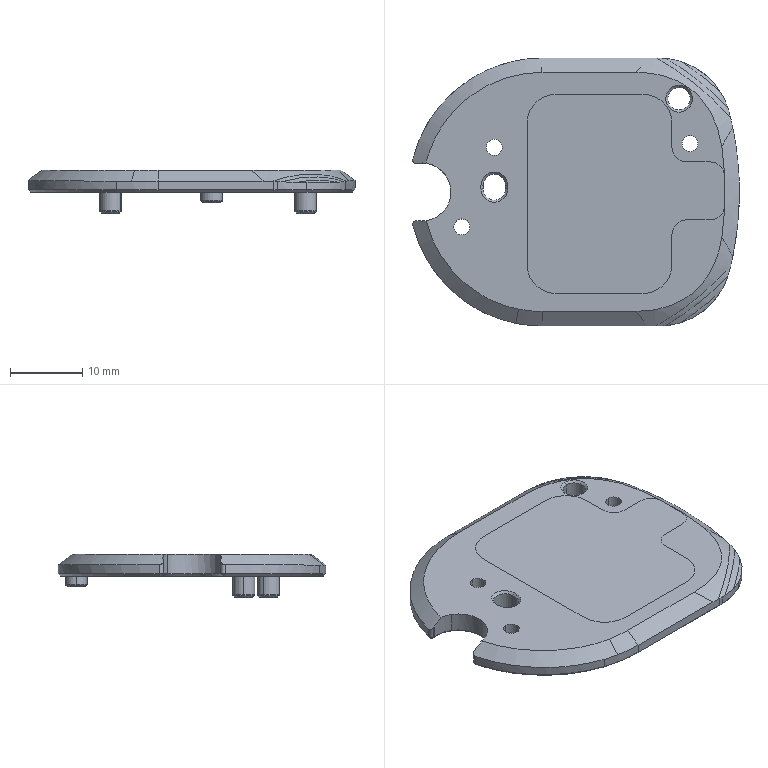NC program | NX | posted with a generic post | part box 45.101 x 36.973 x 6 mm
Lines 1 to 931 of 3161:
N10 G17 G21 G94 G90
(FLOOR_WALL_COPY , TOOL : D80)
N12 T19 M6
N14 G54
N16 G17 G0 G90 X-69.55 Y0. S6500 M3
N18 G43 Z30. H19
N20 Z3.
N22 G94 G1 Z0. F1500.
N24 X-64.55
N26 X64.55
N28 X69.55
N30 Z3.
N32 G0 Z30.
N34 M5
(ZLEVEL_PROFILE , TOOL : D10)
N36 T15 M6
N38 G54
N40 G17 G0 G90 X27.158 Y6.961 S9500 M3
N42 G43 Z30. H15
N44 Z1.5
N46 G94 G1 X27.257 Y6.402 Z1.47 F1000.
N48 X27.633 Y2.132 Z1.245
N50 X27.634 Y-2.155 Z1.021
N52 X27.259 Y-6.426 Z0.796
N54 X26.512 Y-10.647 Z0.571
N56 X26.081 Y-12.305 Z0.482
N58 X25.842 Y-13.227 Z0.432
N60 X24.998 Y-15.279 Z0.315
N62 X23.863 Y-17.185 Z0.199
N64 X22.461 Y-18.904 Z0.083
N66 X20.823 Y-20.4 Z-0.033
N68 X18.984 Y-21.641 Z-0.15
N70 X18.089 Y-22.081 Z-0.202
N72 X17.231 Y-22.495 Z-0.252
N74 X15.107 Y-23.182 Z-0.369
N76 X12.906 Y-23.549 Z-0.486
N78 X11.954 Y-23.576 Z-0.536
N80 X11.298 Y-23.585 Z-0.57
N82 X3.09 Z-1.
N84 X-5.774 Y-23.586 F3200.
N86 G2 X-27.477 Y-5.824 R23.6
N88 X-25.478 Y-0.018 R5.6
N90 X-27.478 Y5.788 R5.6
N92 X-4.605 Y23.585 R23.6
N94 G1 X11.247 Y23.586
N96 G2 X11.845 Y23.579 R23.599
N98 X26.079 Y12.281 R15.1
N100 X26.081 Y-12.305 R48.901
N102 X18.089 Y-22.081 R15.1
N104 X11.954 Y-23.576 R15.1
N106 G1 X11.298 Y-23.585
N108 X3.09
N110 X-4.652 Y-23.586 Z-1.135
N112 X-5.039 Y-23.582 Z-1.142
N114 X-5.426 Y-23.575 Z-1.149
N116 X-5.812 Y-23.559 Z-1.156
N118 X-6.198 Y-23.538 Z-1.162
N120 X-6.584 Y-23.51 Z-1.169
N122 X-6.969 Y-23.476 Z-1.176
N124 X-7.353 Y-23.435 Z-1.183
N126 X-7.737 Y-23.388 Z-1.189
N128 X-8.12 Y-23.335 Z-1.196
N130 X-8.503 Y-23.276 Z-1.203
N132 X-8.884 Y-23.21 Z-1.21
N134 X-9.264 Y-23.138 Z-1.216
N136 X-9.643 Y-23.059 Z-1.223
N138 X-10.021 Y-22.975 Z-1.23
N140 X-10.397 Y-22.885 Z-1.237
N142 X-10.771 Y-22.788 Z-1.243
N144 X-11.145 Y-22.687 Z-1.25
N146 X-11.511 Y-22.56 Z-1.257
N148 X-11.886 Y-22.462 Z-1.264
N150 X-12.253 Y-22.341 Z-1.27
N152 X-12.619 Y-22.213 Z-1.277
N154 X-12.982 Y-22.078 Z-1.284
N156 X-13.342 Y-21.938 Z-1.291
N158 X-13.701 Y-21.791 Z-1.297
N160 X-14.057 Y-21.639 Z-1.304
N162 X-14.41 Y-21.481 Z-1.311
N164 X-14.761 Y-21.318 Z-1.318
N166 X-15.109 Y-21.148 Z-1.325
N168 X-15.454 Y-20.973 Z-1.331
N170 X-15.796 Y-20.792 Z-1.338
N172 X-16.135 Y-20.606 Z-1.345
N174 X-16.472 Y-20.414 Z-1.352
N176 X-16.805 Y-20.216 Z-1.358
N178 X-17.134 Y-20.014 Z-1.365
N180 X-17.461 Y-19.805 Z-1.372
N182 X-17.783 Y-19.592 Z-1.379
N184 X-18.103 Y-19.373 Z-1.385
N186 X-18.418 Y-19.149 Z-1.392
N188 X-18.73 Y-18.92 Z-1.399
N190 X-19.039 Y-18.686 Z-1.406
N192 X-19.343 Y-18.446 Z-1.412
N194 X-19.643 Y-18.202 Z-1.419
N196 X-19.939 Y-17.953 Z-1.426
N198 X-20.232 Y-17.699 Z-1.433
N200 X-20.52 Y-17.44 Z-1.439
N202 X-20.803 Y-17.177 Z-1.446
N204 X-21.082 Y-16.909 Z-1.453
N206 X-21.357 Y-16.636 Z-1.46
N208 X-21.628 Y-16.359 Z-1.466
N210 X-21.893 Y-16.078 Z-1.473
N212 X-22.155 Y-15.792 Z-1.48
N214 X-22.411 Y-15.502 Z-1.487
N216 X-22.663 Y-15.208 Z-1.493
N218 X-22.909 Y-14.91 Z-1.5
N220 X-23.151 Y-14.607 Z-1.507
N222 X-23.388 Y-14.301 Z-1.514
N224 X-23.62 Y-13.991 Z-1.52
N226 X-23.846 Y-13.677 Z-1.527
N228 X-24.068 Y-13.36 Z-1.534
N230 X-24.284 Y-13.039 Z-1.541
N232 X-24.495 Y-12.714 Z-1.547
N234 X-24.701 Y-12.386 Z-1.554
N236 X-24.901 Y-12.055 Z-1.561
N238 X-25.096 Y-11.721 Z-1.568
N240 X-25.285 Y-11.383 Z-1.575
N242 X-25.469 Y-11.042 Z-1.581
N244 X-25.647 Y-10.698 Z-1.588
N246 X-25.819 Y-10.352 Z-1.595
N248 X-25.986 Y-10.003 Z-1.602
N250 X-26.147 Y-9.65 Z-1.608
N252 X-26.302 Y-9.296 Z-1.615
N254 X-26.451 Y-8.939 Z-1.622
N256 X-26.595 Y-8.579 Z-1.629
N258 X-26.732 Y-8.217 Z-1.635
N260 X-26.864 Y-7.853 Z-1.642
N262 X-26.989 Y-7.487 Z-1.649
N264 X-27.109 Y-7.119 Z-1.656
N266 X-27.222 Y-6.749 Z-1.662
N268 X-27.33 Y-6.377 Z-1.669
N270 X-27.431 Y-6.003 Z-1.676
N272 X-27.523 Y-5.627 Z-1.683
N274 X-27.592 Y-5.247 Z-1.689
N276 X-27.634 Y-4.862 Z-1.696
N278 X-27.649 Y-4.475 Z-1.703
N280 X-27.638 Y-4.088 Z-1.71
N282 X-27.6 Y-3.703 Z-1.716
N284 X-27.535 Y-3.322 Z-1.723
N286 X-27.445 Y-2.945 Z-1.73
N288 X-27.328 Y-2.576 Z-1.737
N290 X-27.186 Y-2.216 Z-1.743
N292 X-27.02 Y-1.867 Z-1.75
N294 X-26.83 Y-1.53 Z-1.757
N296 X-26.617 Y-1.206 Z-1.764
N298 X-26.383 Y-0.899 Z-1.77
N300 X-26.127 Y-0.608 Z-1.777
N302 X-25.852 Y-0.335 Z-1.784
N304 X-25.487 Y-0.009 Z-1.793
N306 X-25.697 Y0.161 Z-1.797
N308 X-25.982 Y0.423 Z-1.804
N310 X-26.248 Y0.704 Z-1.811
N312 X-26.494 Y1.003 Z-1.818
N314 X-26.718 Y1.318 Z-1.825
N316 X-26.921 Y1.648 Z-1.831
N318 X-27.1 Y1.991 Z-1.838
N320 X-27.255 Y2.345 Z-1.845
N322 X-27.386 Y2.71 Z-1.852
N324 X-27.49 Y3.082 Z-1.858
N326 X-27.569 Y3.461 Z-1.865
N328 X-27.622 Y3.844 Z-1.872
N330 X-27.647 Y4.231 Z-1.879
N332 Y4.618 Z-1.885
N334 X-27.619 Y5.004 Z-1.892
N336 X-27.565 Y5.387 Z-1.899
N338 X-27.484 Y5.765 Z-1.906
N340 X-27.386 Y6.14 Z-1.912
N342 X-27.282 Y6.513 Z-1.919
N344 X-27.172 Y6.884 Z-1.926
N346 X-27.056 Y7.253 Z-1.933
N348 X-26.934 Y7.62 Z-1.939
N350 X-26.805 Y7.986 Z-1.946
N352 X-26.671 Y8.349 Z-1.953
N354 X-26.531 Y8.71 Z-1.96
N356 X-26.385 Y9.068 Z-1.966
N358 X-26.233 Y9.424 Z-1.973
N360 X-26.075 Y9.778 Z-1.98
N362 X-25.912 Y10.128 Z-1.987
N364 X-25.743 Y10.477 Z-1.993
N366 X-25.568 Y10.822 Z-2.
N368 G2 X-4.605 Y23.585 R23.6
N370 G1 X11.247 Y23.586
N372 G2 X11.845 Y23.579 R23.599
N374 X26.079 Y12.281 R15.1
N376 X26.081 Y-12.305 R48.901
N378 X18.089 Y-22.081 R15.1
N380 X11.954 Y-23.576 R15.1
N382 G1 X11.298 Y-23.585
N384 X3.09
N386 X-4.652 Y-23.586 Z-2.135
N388 X-5.039 Y-23.582 Z-2.142
N390 X-5.426 Y-23.575 Z-2.149
N392 X-5.812 Y-23.559 Z-2.156
N394 X-6.198 Y-23.538 Z-2.162
N396 X-6.584 Y-23.51 Z-2.169
N398 X-6.969 Y-23.476 Z-2.176
N400 X-7.353 Y-23.435 Z-2.183
N402 X-7.737 Y-23.388 Z-2.189
N404 X-8.12 Y-23.335 Z-2.196
N406 X-8.503 Y-23.276 Z-2.203
N408 X-8.884 Y-23.21 Z-2.21
N410 X-9.264 Y-23.138 Z-2.216
N412 X-9.643 Y-23.059 Z-2.223
N414 X-10.021 Y-22.975 Z-2.23
N416 X-10.397 Y-22.885 Z-2.237
N418 X-10.771 Y-22.788 Z-2.243
N420 X-11.145 Y-22.687 Z-2.25
N422 X-11.511 Y-22.56 Z-2.257
N424 X-11.886 Y-22.462 Z-2.264
N426 X-12.253 Y-22.341 Z-2.27
N428 X-12.619 Y-22.213 Z-2.277
N430 X-12.982 Y-22.078 Z-2.284
N432 X-13.342 Y-21.938 Z-2.291
N434 X-13.701 Y-21.791 Z-2.297
N436 X-14.057 Y-21.639 Z-2.304
N438 X-14.41 Y-21.481 Z-2.311
N440 X-14.761 Y-21.318 Z-2.318
N442 X-15.109 Y-21.148 Z-2.325
N444 X-15.454 Y-20.973 Z-2.331
N446 X-15.796 Y-20.792 Z-2.338
N448 X-16.135 Y-20.606 Z-2.345
N450 X-16.472 Y-20.414 Z-2.352
N452 X-16.805 Y-20.216 Z-2.358
N454 X-17.134 Y-20.014 Z-2.365
N456 X-17.461 Y-19.805 Z-2.372
N458 X-17.783 Y-19.592 Z-2.379
N460 X-18.103 Y-19.373 Z-2.385
N462 X-18.418 Y-19.149 Z-2.392
N464 X-18.73 Y-18.92 Z-2.399
N466 X-19.039 Y-18.686 Z-2.406
N468 X-19.343 Y-18.446 Z-2.412
N470 X-19.643 Y-18.202 Z-2.419
N472 X-19.939 Y-17.953 Z-2.426
N474 X-20.232 Y-17.699 Z-2.433
N476 X-20.52 Y-17.44 Z-2.439
N478 X-20.803 Y-17.177 Z-2.446
N480 X-21.082 Y-16.909 Z-2.453
N482 X-21.357 Y-16.636 Z-2.46
N484 X-21.628 Y-16.359 Z-2.466
N486 X-21.893 Y-16.078 Z-2.473
N488 X-22.155 Y-15.792 Z-2.48
N490 X-22.411 Y-15.502 Z-2.487
N492 X-22.663 Y-15.208 Z-2.493
N494 X-22.909 Y-14.91 Z-2.5
N496 X-23.151 Y-14.607 Z-2.507
N498 X-23.388 Y-14.301 Z-2.514
N500 X-23.62 Y-13.991 Z-2.52
N502 X-23.846 Y-13.677 Z-2.527
N504 X-24.068 Y-13.36 Z-2.534
N506 X-24.284 Y-13.039 Z-2.541
N508 X-24.495 Y-12.714 Z-2.547
N510 X-24.701 Y-12.386 Z-2.554
N512 X-24.901 Y-12.055 Z-2.561
N514 X-25.096 Y-11.721 Z-2.568
N516 X-25.285 Y-11.383 Z-2.575
N518 X-25.469 Y-11.042 Z-2.581
N520 X-25.647 Y-10.698 Z-2.588
N522 X-25.819 Y-10.352 Z-2.595
N524 X-25.986 Y-10.003 Z-2.602
N526 X-26.147 Y-9.65 Z-2.608
N528 X-26.302 Y-9.296 Z-2.615
N530 X-26.451 Y-8.939 Z-2.622
N532 X-26.595 Y-8.579 Z-2.629
N534 X-26.732 Y-8.217 Z-2.635
N536 X-26.864 Y-7.853 Z-2.642
N538 X-26.989 Y-7.487 Z-2.649
N540 X-27.109 Y-7.119 Z-2.656
N542 X-27.222 Y-6.749 Z-2.662
N544 X-27.33 Y-6.377 Z-2.669
N546 X-27.431 Y-6.003 Z-2.676
N548 X-27.523 Y-5.627 Z-2.683
N550 X-27.592 Y-5.247 Z-2.689
N552 X-27.634 Y-4.862 Z-2.696
N554 X-27.649 Y-4.475 Z-2.703
N556 X-27.638 Y-4.088 Z-2.71
N558 X-27.6 Y-3.703 Z-2.716
N560 X-27.535 Y-3.322 Z-2.723
N562 X-27.445 Y-2.945 Z-2.73
N564 X-27.328 Y-2.576 Z-2.737
N566 X-27.186 Y-2.216 Z-2.743
N568 X-27.02 Y-1.867 Z-2.75
N570 X-26.83 Y-1.53 Z-2.757
N572 X-26.617 Y-1.206 Z-2.764
N574 X-26.383 Y-0.899 Z-2.77
N576 X-26.127 Y-0.608 Z-2.777
N578 X-25.852 Y-0.335 Z-2.784
N580 X-25.487 Y-0.009 Z-2.793
N582 X-25.697 Y0.161 Z-2.797
N584 X-25.982 Y0.423 Z-2.804
N586 X-26.248 Y0.704 Z-2.811
N588 X-26.494 Y1.003 Z-2.818
N590 X-26.718 Y1.318 Z-2.825
N592 X-26.921 Y1.648 Z-2.831
N594 X-27.1 Y1.991 Z-2.838
N596 X-27.255 Y2.345 Z-2.845
N598 X-27.386 Y2.71 Z-2.852
N600 X-27.49 Y3.082 Z-2.858
N602 X-27.569 Y3.461 Z-2.865
N604 X-27.622 Y3.844 Z-2.872
N606 X-27.647 Y4.231 Z-2.879
N608 Y4.618 Z-2.885
N610 X-27.619 Y5.004 Z-2.892
N612 X-27.565 Y5.387 Z-2.899
N614 X-27.484 Y5.765 Z-2.906
N616 X-27.386 Y6.14 Z-2.912
N618 X-27.282 Y6.513 Z-2.919
N620 X-27.172 Y6.884 Z-2.926
N622 X-27.056 Y7.253 Z-2.933
N624 X-26.934 Y7.62 Z-2.939
N626 X-26.805 Y7.986 Z-2.946
N628 X-26.671 Y8.349 Z-2.953
N630 X-26.531 Y8.71 Z-2.96
N632 X-26.385 Y9.068 Z-2.966
N634 X-26.233 Y9.424 Z-2.973
N636 X-26.075 Y9.778 Z-2.98
N638 X-25.912 Y10.128 Z-2.987
N640 X-25.743 Y10.477 Z-2.993
N642 X-25.568 Y10.822 Z-3.
N644 G2 X-4.605 Y23.585 R23.6
N646 G1 X11.247 Y23.586
N648 G2 X11.845 Y23.579 R23.599
N650 X26.079 Y12.281 R15.1
N652 X26.081 Y-12.305 R48.901
N654 X18.089 Y-22.081 R15.1
N656 X11.954 Y-23.576 R15.1
N658 G1 X11.298 Y-23.585
N660 X3.09
N662 X-4.652 Y-23.586 Z-3.135
N664 X-5.039 Y-23.582 Z-3.142
N666 X-5.426 Y-23.575 Z-3.149
N668 X-5.812 Y-23.559 Z-3.156
N670 X-6.198 Y-23.538 Z-3.162
N672 X-6.584 Y-23.51 Z-3.169
N674 X-6.969 Y-23.476 Z-3.176
N676 X-7.353 Y-23.435 Z-3.183
N678 X-7.737 Y-23.388 Z-3.189
N680 X-8.12 Y-23.335 Z-3.196
N682 X-8.503 Y-23.276 Z-3.203
N684 X-8.884 Y-23.21 Z-3.21
N686 X-9.264 Y-23.138 Z-3.216
N688 X-9.643 Y-23.059 Z-3.223
N690 X-10.021 Y-22.975 Z-3.23
N692 X-10.397 Y-22.885 Z-3.237
N694 X-10.771 Y-22.788 Z-3.243
N696 X-11.145 Y-22.687 Z-3.25
N698 X-11.511 Y-22.56 Z-3.257
N700 X-11.886 Y-22.462 Z-3.264
N702 X-12.253 Y-22.341 Z-3.27
N704 X-12.619 Y-22.213 Z-3.277
N706 X-12.982 Y-22.078 Z-3.284
N708 X-13.342 Y-21.938 Z-3.291
N710 X-13.701 Y-21.791 Z-3.297
N712 X-14.057 Y-21.639 Z-3.304
N714 X-14.41 Y-21.481 Z-3.311
N716 X-14.761 Y-21.318 Z-3.318
N718 X-15.109 Y-21.148 Z-3.325
N720 X-15.454 Y-20.973 Z-3.331
N722 X-15.796 Y-20.792 Z-3.338
N724 X-16.135 Y-20.606 Z-3.345
N726 X-16.472 Y-20.414 Z-3.352
N728 X-16.805 Y-20.216 Z-3.358
N730 X-17.134 Y-20.014 Z-3.365
N732 X-17.461 Y-19.805 Z-3.372
N734 X-17.783 Y-19.592 Z-3.379
N736 X-18.103 Y-19.373 Z-3.385
N738 X-18.418 Y-19.149 Z-3.392
N740 X-18.73 Y-18.92 Z-3.399
N742 X-19.039 Y-18.686 Z-3.406
N744 X-19.343 Y-18.446 Z-3.412
N746 X-19.643 Y-18.202 Z-3.419
N748 X-19.939 Y-17.953 Z-3.426
N750 X-20.232 Y-17.699 Z-3.433
N752 X-20.52 Y-17.44 Z-3.439
N754 X-20.803 Y-17.177 Z-3.446
N756 X-21.082 Y-16.909 Z-3.453
N758 X-21.357 Y-16.636 Z-3.46
N760 X-21.628 Y-16.359 Z-3.466
N762 X-21.893 Y-16.078 Z-3.473
N764 X-22.155 Y-15.792 Z-3.48
N766 X-22.411 Y-15.502 Z-3.487
N768 X-22.663 Y-15.208 Z-3.493
N770 X-22.909 Y-14.91 Z-3.5
N772 X-23.151 Y-14.607 Z-3.507
N774 X-23.388 Y-14.301 Z-3.514
N776 X-23.62 Y-13.991 Z-3.52
N778 X-23.846 Y-13.677 Z-3.527
N780 X-24.068 Y-13.36 Z-3.534
N782 X-24.284 Y-13.039 Z-3.541
N784 X-24.495 Y-12.714 Z-3.547
N786 X-24.701 Y-12.386 Z-3.554
N788 X-24.901 Y-12.055 Z-3.561
N790 X-25.096 Y-11.721 Z-3.568
N792 X-25.285 Y-11.383 Z-3.575
N794 X-25.469 Y-11.042 Z-3.581
N796 X-25.647 Y-10.698 Z-3.588
N798 X-25.819 Y-10.352 Z-3.595
N800 X-25.986 Y-10.003 Z-3.602
N802 X-26.147 Y-9.65 Z-3.608
N804 X-26.302 Y-9.296 Z-3.615
N806 X-26.451 Y-8.939 Z-3.622
N808 X-26.595 Y-8.579 Z-3.629
N810 X-26.732 Y-8.217 Z-3.635
N812 X-26.864 Y-7.853 Z-3.642
N814 X-26.989 Y-7.487 Z-3.649
N816 X-27.109 Y-7.119 Z-3.656
N818 X-27.222 Y-6.749 Z-3.662
N820 X-27.33 Y-6.377 Z-3.669
N822 X-27.431 Y-6.003 Z-3.676
N824 X-27.523 Y-5.627 Z-3.683
N826 X-27.592 Y-5.247 Z-3.689
N828 X-27.634 Y-4.862 Z-3.696
N830 X-27.649 Y-4.475 Z-3.703
N832 X-27.638 Y-4.088 Z-3.71
N834 X-27.6 Y-3.703 Z-3.716
N836 X-27.535 Y-3.322 Z-3.723
N838 X-27.445 Y-2.945 Z-3.73
N840 X-27.328 Y-2.576 Z-3.737
N842 X-27.186 Y-2.216 Z-3.743
N844 X-27.02 Y-1.867 Z-3.75
N846 X-26.83 Y-1.53 Z-3.757
N848 X-26.617 Y-1.206 Z-3.764
N850 X-26.383 Y-0.899 Z-3.77
N852 X-26.127 Y-0.608 Z-3.777
N854 X-25.852 Y-0.335 Z-3.784
N856 X-25.487 Y-0.009 Z-3.793
N858 X-25.697 Y0.161 Z-3.797
N860 X-25.982 Y0.423 Z-3.804
N862 X-26.248 Y0.704 Z-3.811
N864 X-26.494 Y1.003 Z-3.818
N866 X-26.718 Y1.318 Z-3.825
N868 X-26.921 Y1.648 Z-3.831
N870 X-27.1 Y1.991 Z-3.838
N872 X-27.255 Y2.345 Z-3.845
N874 X-27.386 Y2.71 Z-3.852
N876 X-27.49 Y3.082 Z-3.858
N878 X-27.569 Y3.461 Z-3.865
N880 X-27.622 Y3.844 Z-3.872
N882 X-27.647 Y4.231 Z-3.879
N884 Y4.618 Z-3.885
N886 X-27.619 Y5.004 Z-3.892
N888 X-27.565 Y5.387 Z-3.899
N890 X-27.484 Y5.765 Z-3.906
N892 X-27.386 Y6.14 Z-3.912
N894 X-27.282 Y6.513 Z-3.919
N896 X-27.172 Y6.884 Z-3.926
N898 X-27.056 Y7.253 Z-3.933
N900 X-26.934 Y7.62 Z-3.939
N902 X-26.805 Y7.986 Z-3.946
N904 X-26.671 Y8.349 Z-3.953
N906 X-26.531 Y8.71 Z-3.96
N908 X-26.385 Y9.068 Z-3.966
N910 X-26.233 Y9.424 Z-3.973
N912 X-26.075 Y9.778 Z-3.98
N914 X-25.912 Y10.128 Z-3.987
N916 X-25.743 Y10.477 Z-3.993
N918 X-25.568 Y10.822 Z-4.
N920 G2 X-4.605 Y23.585 R23.6
N922 G1 X11.247 Y23.586
N924 G2 X11.845 Y23.579 R23.599
N926 X26.079 Y12.281 R15.1
N928 X26.081 Y-12.305 R48.901
N930 X18.089 Y-22.081 R15.1
N932 X11.954 Y-23.576 R15.1
N934 G1 X11.298 Y-23.585
N936 X3.09
N938 X-4.652 Y-23.586 Z-4.135
N940 X-5.039 Y-23.582 Z-4.142
N942 X-5.426 Y-23.575 Z-4.149
N944 X-5.812 Y-23.559 Z-4.156
N946 X-6.198 Y-23.538 Z-4.162
N948 X-6.584 Y-23.51 Z-4.169
N950 X-6.969 Y-23.476 Z-4.176
N952 X-7.353 Y-23.435 Z-4.183
N954 X-7.737 Y-23.388 Z-4.189
N956 X-8.12 Y-23.335 Z-4.196
N958 X-8.503 Y-23.276 Z-4.203
N960 X-8.884 Y-23.21 Z-4.21
N962 X-9.264 Y-23.138 Z-4.216
N964 X-9.643 Y-23.059 Z-4.223
N966 X-10.021 Y-22.975 Z-4.23
N968 X-10.397 Y-22.885 Z-4.237
N970 X-10.771 Y-22.788 Z-4.243
N972 X-11.145 Y-22.687 Z-4.25
N974 X-11.511 Y-22.56 Z-4.257
N976 X-11.886 Y-22.462 Z-4.264
N978 X-12.253 Y-22.341 Z-4.27
N980 X-12.619 Y-22.213 Z-4.277
N982 X-12.982 Y-22.078 Z-4.284
N984 X-13.342 Y-21.938 Z-4.291
N986 X-13.701 Y-21.791 Z-4.297
N988 X-14.057 Y-21.639 Z-4.304
N990 X-14.41 Y-21.481 Z-4.311
N992 X-14.761 Y-21.318 Z-4.318
N994 X-15.109 Y-21.148 Z-4.325
N996 X-15.454 Y-20.973 Z-4.331
N998 X-15.796 Y-20.792 Z-4.338
N1000 X-16.135 Y-20.606 Z-4.345
N1002 X-16.472 Y-20.414 Z-4.352
N1004 X-16.805 Y-20.216 Z-4.358
N1006 X-17.134 Y-20.014 Z-4.365
N1008 X-17.461 Y-19.805 Z-4.372
N1010 X-17.783 Y-19.592 Z-4.379
N1012 X-18.103 Y-19.373 Z-4.385
N1014 X-18.418 Y-19.149 Z-4.392
N1016 X-18.73 Y-18.92 Z-4.399
N1018 X-19.039 Y-18.686 Z-4.406
N1020 X-19.343 Y-18.446 Z-4.412
N1022 X-19.643 Y-18.202 Z-4.419
N1024 X-19.939 Y-17.953 Z-4.426
N1026 X-20.232 Y-17.699 Z-4.433
N1028 X-20.52 Y-17.44 Z-4.439
N1030 X-20.803 Y-17.177 Z-4.446
N1032 X-21.082 Y-16.909 Z-4.453
N1034 X-21.357 Y-16.636 Z-4.46
N1036 X-21.628 Y-16.359 Z-4.466
N1038 X-21.893 Y-16.078 Z-4.473
N1040 X-22.155 Y-15.792 Z-4.48
N1042 X-22.411 Y-15.502 Z-4.487
N1044 X-22.663 Y-15.208 Z-4.493
N1046 X-22.909 Y-14.91 Z-4.5
N1048 X-23.151 Y-14.607 Z-4.507
N1050 X-23.388 Y-14.301 Z-4.514
N1052 X-23.62 Y-13.991 Z-4.52
N1054 X-23.846 Y-13.677 Z-4.527
N1056 X-24.068 Y-13.36 Z-4.534
N1058 X-24.284 Y-13.039 Z-4.541
N1060 X-24.495 Y-12.714 Z-4.547
N1062 X-24.701 Y-12.386 Z-4.554
N1064 X-24.901 Y-12.055 Z-4.561
N1066 X-25.096 Y-11.721 Z-4.568
N1068 X-25.285 Y-11.383 Z-4.575
N1070 X-25.469 Y-11.042 Z-4.581
N1072 X-25.647 Y-10.698 Z-4.588
N1074 X-25.819 Y-10.352 Z-4.595
N1076 X-25.986 Y-10.003 Z-4.602
N1078 X-26.147 Y-9.65 Z-4.608
N1080 X-26.302 Y-9.296 Z-4.615
N1082 X-26.451 Y-8.939 Z-4.622
N1084 X-26.595 Y-8.579 Z-4.629
N1086 X-26.732 Y-8.217 Z-4.635
N1088 X-26.864 Y-7.853 Z-4.642
N1090 X-26.989 Y-7.487 Z-4.649
N1092 X-27.109 Y-7.119 Z-4.656
N1094 X-27.222 Y-6.749 Z-4.662
N1096 X-27.33 Y-6.377 Z-4.669
N1098 X-27.431 Y-6.003 Z-4.676
N1100 X-27.523 Y-5.627 Z-4.683
N1102 X-27.592 Y-5.247 Z-4.689
N1104 X-27.634 Y-4.862 Z-4.696
N1106 X-27.649 Y-4.475 Z-4.703
N1108 X-27.638 Y-4.088 Z-4.71
N1110 X-27.6 Y-3.703 Z-4.716
N1112 X-27.535 Y-3.322 Z-4.723
N1114 X-27.445 Y-2.945 Z-4.73
N1116 X-27.328 Y-2.576 Z-4.737
N1118 X-27.186 Y-2.216 Z-4.743
N1120 X-27.02 Y-1.867 Z-4.75
N1122 X-26.83 Y-1.53 Z-4.757
N1124 X-26.617 Y-1.206 Z-4.764
N1126 X-26.383 Y-0.899 Z-4.77
N1128 X-26.127 Y-0.608 Z-4.777
N1130 X-25.852 Y-0.335 Z-4.784
N1132 X-25.487 Y-0.009 Z-4.793
N1134 X-25.697 Y0.161 Z-4.797
N1136 X-25.982 Y0.423 Z-4.804
N1138 X-26.248 Y0.704 Z-4.811
N1140 X-26.494 Y1.003 Z-4.818
N1142 X-26.718 Y1.318 Z-4.825
N1144 X-26.921 Y1.648 Z-4.831
N1146 X-27.1 Y1.991 Z-4.838
N1148 X-27.255 Y2.345 Z-4.845
N1150 X-27.386 Y2.71 Z-4.852
N1152 X-27.49 Y3.082 Z-4.858
N1154 X-27.569 Y3.461 Z-4.865
N1156 X-27.622 Y3.844 Z-4.872
N1158 X-27.647 Y4.231 Z-4.879
N1160 Y4.618 Z-4.885
N1162 X-27.619 Y5.004 Z-4.892
N1164 X-27.565 Y5.387 Z-4.899
N1166 X-27.484 Y5.765 Z-4.906
N1168 X-27.386 Y6.14 Z-4.912
N1170 X-27.282 Y6.513 Z-4.919
N1172 X-27.172 Y6.884 Z-4.926
N1174 X-27.056 Y7.253 Z-4.933
N1176 X-26.934 Y7.62 Z-4.939
N1178 X-26.805 Y7.986 Z-4.946
N1180 X-26.671 Y8.349 Z-4.953
N1182 X-26.531 Y8.71 Z-4.96
N1184 X-26.385 Y9.068 Z-4.966
N1186 X-26.233 Y9.424 Z-4.973
N1188 X-26.075 Y9.778 Z-4.98
N1190 X-25.912 Y10.128 Z-4.987
N1192 X-25.743 Y10.477 Z-4.993
N1194 X-25.568 Y10.822 Z-5.
N1196 G2 X-4.605 Y23.585 R23.6
N1198 G1 X11.247 Y23.586
N1200 G2 X11.845 Y23.579 R23.599
N1202 X26.079 Y12.281 R15.1
N1204 X26.081 Y-12.305 R48.901
N1206 X18.089 Y-22.081 R15.1
N1208 X11.954 Y-23.576 R15.1
N1210 G1 X11.298 Y-23.585
N1212 X3.09
N1214 X-4.652 Y-23.586 Z-5.135
N1216 X-5.039 Y-23.582 Z-5.142
N1218 X-5.426 Y-23.575 Z-5.149
N1220 X-5.812 Y-23.559 Z-5.156
N1222 X-6.198 Y-23.538 Z-5.162
N1224 X-6.584 Y-23.51 Z-5.169
N1226 X-6.969 Y-23.476 Z-5.176
N1228 X-7.353 Y-23.435 Z-5.183
N1230 X-7.737 Y-23.388 Z-5.189
N1232 X-8.12 Y-23.335 Z-5.196
N1234 X-8.503 Y-23.276 Z-5.203
N1236 X-8.884 Y-23.21 Z-5.21
N1238 X-9.264 Y-23.138 Z-5.216
N1240 X-9.643 Y-23.059 Z-5.223
N1242 X-10.021 Y-22.975 Z-5.23
N1244 X-10.397 Y-22.885 Z-5.237
N1246 X-10.771 Y-22.788 Z-5.243
N1248 X-11.145 Y-22.687 Z-5.25
N1250 X-11.511 Y-22.56 Z-5.257
N1252 X-11.886 Y-22.462 Z-5.264
N1254 X-12.253 Y-22.341 Z-5.27
N1256 X-12.619 Y-22.213 Z-5.277
N1258 X-12.982 Y-22.078 Z-5.284
N1260 X-13.342 Y-21.938 Z-5.291
N1262 X-13.701 Y-21.791 Z-5.297
N1264 X-14.057 Y-21.639 Z-5.304
N1266 X-14.41 Y-21.481 Z-5.311
N1268 X-14.761 Y-21.318 Z-5.318
N1270 X-15.109 Y-21.148 Z-5.325
N1272 X-15.454 Y-20.973 Z-5.331
N1274 X-15.796 Y-20.792 Z-5.338
N1276 X-16.135 Y-20.606 Z-5.345
N1278 X-16.472 Y-20.414 Z-5.352
N1280 X-16.805 Y-20.216 Z-5.358
N1282 X-17.134 Y-20.014 Z-5.365
N1284 X-17.461 Y-19.805 Z-5.372
N1286 X-17.783 Y-19.592 Z-5.379
N1288 X-18.103 Y-19.373 Z-5.385
N1290 X-18.418 Y-19.149 Z-5.392
N1292 X-18.73 Y-18.92 Z-5.399
N1294 X-19.039 Y-18.686 Z-5.406
N1296 X-19.343 Y-18.446 Z-5.412
N1298 X-19.643 Y-18.202 Z-5.419
N1300 X-19.939 Y-17.953 Z-5.426
N1302 X-20.232 Y-17.699 Z-5.433
N1304 X-20.52 Y-17.44 Z-5.439
N1306 X-20.803 Y-17.177 Z-5.446
N1308 X-21.082 Y-16.909 Z-5.453
N1310 X-21.357 Y-16.636 Z-5.46
N1312 X-21.628 Y-16.359 Z-5.466
N1314 X-21.893 Y-16.078 Z-5.473
N1316 X-22.155 Y-15.792 Z-5.48
N1318 X-22.411 Y-15.502 Z-5.487
N1320 X-22.663 Y-15.208 Z-5.493
N1322 X-22.909 Y-14.91 Z-5.5
N1324 X-23.151 Y-14.607 Z-5.507
N1326 X-23.388 Y-14.301 Z-5.514
N1328 X-23.62 Y-13.991 Z-5.52
N1330 X-23.846 Y-13.677 Z-5.527
N1332 X-24.068 Y-13.36 Z-5.534
N1334 X-24.284 Y-13.039 Z-5.541
N1336 X-24.495 Y-12.714 Z-5.547
N1338 X-24.701 Y-12.386 Z-5.554
N1340 X-24.901 Y-12.055 Z-5.561
N1342 X-25.096 Y-11.721 Z-5.568
N1344 X-25.285 Y-11.383 Z-5.575
N1346 X-25.469 Y-11.042 Z-5.581
N1348 X-25.647 Y-10.698 Z-5.588
N1350 X-25.819 Y-10.352 Z-5.595
N1352 X-25.986 Y-10.003 Z-5.602
N1354 X-26.147 Y-9.65 Z-5.608
N1356 X-26.302 Y-9.296 Z-5.615
N1358 X-26.451 Y-8.939 Z-5.622
N1360 X-26.595 Y-8.579 Z-5.629
N1362 X-26.732 Y-8.217 Z-5.635
N1364 X-26.864 Y-7.853 Z-5.642
N1366 X-26.989 Y-7.487 Z-5.649
N1368 X-27.109 Y-7.119 Z-5.656
N1370 X-27.222 Y-6.749 Z-5.662
N1372 X-27.33 Y-6.377 Z-5.669
N1374 X-27.431 Y-6.003 Z-5.676
N1376 X-27.523 Y-5.627 Z-5.683
N1378 X-27.592 Y-5.247 Z-5.689
N1380 X-27.634 Y-4.862 Z-5.696
N1382 X-27.649 Y-4.475 Z-5.703
N1384 X-27.638 Y-4.088 Z-5.71
N1386 X-27.6 Y-3.703 Z-5.716
N1388 X-27.535 Y-3.322 Z-5.723
N1390 X-27.445 Y-2.945 Z-5.73
N1392 X-27.328 Y-2.576 Z-5.737
N1394 X-27.186 Y-2.216 Z-5.743
N1396 X-27.02 Y-1.867 Z-5.75
N1398 X-26.83 Y-1.53 Z-5.757
N1400 X-26.617 Y-1.206 Z-5.764
N1402 X-26.383 Y-0.899 Z-5.77
N1404 X-26.127 Y-0.608 Z-5.777
N1406 X-25.852 Y-0.335 Z-5.784
N1408 X-25.487 Y-0.009 Z-5.793
N1410 X-25.697 Y0.161 Z-5.797
N1412 X-25.982 Y0.423 Z-5.804
N1414 X-26.248 Y0.704 Z-5.811
N1416 X-26.494 Y1.003 Z-5.818
N1418 X-26.718 Y1.318 Z-5.825
N1420 X-26.921 Y1.648 Z-5.831
N1422 X-27.1 Y1.991 Z-5.838
N1424 X-27.255 Y2.345 Z-5.845
N1426 X-27.386 Y2.71 Z-5.852
N1428 X-27.49 Y3.082 Z-5.858
N1430 X-27.569 Y3.461 Z-5.865
N1432 X-27.622 Y3.844 Z-5.872
N1434 X-27.647 Y4.231 Z-5.879
N1436 Y4.618 Z-5.885
N1438 X-27.619 Y5.004 Z-5.892
N1440 X-27.565 Y5.387 Z-5.899
N1442 X-27.484 Y5.765 Z-5.906
N1444 X-27.386 Y6.14 Z-5.912
N1446 X-27.282 Y6.513 Z-5.919
N1448 X-27.172 Y6.884 Z-5.926
N1450 X-27.056 Y7.253 Z-5.933
N1452 X-26.934 Y7.62 Z-5.939
N1454 X-26.805 Y7.986 Z-5.946
N1456 X-26.671 Y8.349 Z-5.953
N1458 X-26.531 Y8.71 Z-5.96
N1460 X-26.385 Y9.068 Z-5.966
N1462 X-26.233 Y9.424 Z-5.973
N1464 X-26.075 Y9.778 Z-5.98
N1466 X-25.912 Y10.128 Z-5.987
N1468 X-25.743 Y10.477 Z-5.993
N1470 X-25.568 Y10.822 Z-6.
N1472 G2 X-4.605 Y23.585 R23.6
N1474 G1 X11.247 Y23.586
N1476 G2 X11.845 Y23.579 R23.599
N1478 X26.079 Y12.281 R15.1
N1480 X26.081 Y-12.305 R48.901
N1482 X18.089 Y-22.081 R15.1
N1484 X11.954 Y-23.576 R15.1
N1486 G1 X11.298 Y-23.585
N1488 X-5.774 Y-23.586
N1490 G2 X-27.477 Y-5.824 R23.6
N1492 X-25.478 Y-0.018 R5.6
N1494 X-27.478 Y5.788 R5.6
N1496 X-25.568 Y10.822 R23.6
N1498 G1 Z-4.5
N1500 G0 Z30.
N1502 M5
(CAVITY_MILL_COPY , TOOL : D6)
N1504 T12 M6
N1506 G54
N1508 G17 G0 G90 X-25.052 Y-1.732 S9509 M3
N1510 G43 Z30. H12
N1512 Z0.4
N1514 G94 G1 Z-0.6 F1000.
N1516 X-24.237 Y-1.888
N1518 G3 X-23.417 Y-1.681 R1.
N1520 G2 X-21.32 Y-1.015 R2.995 F1800.
N1522 G3 X-20.479 Y0.618 R1.
N1524 X-20.77 Y0.861 R1.001
N1526 X-21.355 Y1.01 R1.
N1528 G2 X-23.459 Y1.71 R2.998
N1530 G3 X-24.275 Y1.93 R1.
N1532 G1 X-25.094 Y1.788
N1534 Z0.4
N1536 G0 X-25.847 Y-1.732 Z-0.2
N1538 G1 Z-1.2 F1000.
N1540 X-25.032 Y-1.895
N1542 G3 X-24.211 Y-1.694 R1.
N1544 G2 X-24.042 Y-1.568 R2.999 F1800.
N1546 X-21.428 Y-1.001 R3.5
N1548 G3 X-20.479 Y0.618 R1.
N1550 X-20.77 Y0.861 R1.001
N1552 X-21.486 Y0.994 R1.
N1554 G2 X-22.61 Y0.964 R3.5
N1556 X-23.155 Y1.09 R3.
N1558 X-24.216 Y1.662 R3.5
N1560 G3 X-25.039 Y1.855 R1.
N1562 G1 X-25.837 Y1.689
N1564 Z-0.2
N1566 G0 X-25.875 Y-1.716 Z-0.8
N1568 G1 Z-1.8 F1000.
N1570 X-25.038 Y-1.89
N1572 G3 X-24.215 Y-1.697 R1.
N1574 G2 X-21.428 Y-1.001 R3.5 F1800.
N1576 G3 X-20.479 Y0.618 R1.
N1578 X-20.77 Y0.861 R1.001
N1580 X-21.486 Y0.994 R1.
N1582 G2 X-22.61 Y0.964 R3.5
N1584 X-23.155 Y1.09 R3.
N1586 X-24.24 Y1.68 R3.5
N1588 G3 X-25.061 Y1.881 R1.
N1590 G1 X-25.899 Y1.714
N1592 Z-0.8
N1594 G0 X-25.875 Y-1.716 Z-1.4
N1596 G1 Z-2.4 F1000.
N1598 X-25.038 Y-1.89
N1600 G3 X-24.215 Y-1.697 R1.
N1602 G2 X-21.428 Y-1.001 R3.5 F1800.
N1604 G3 X-20.479 Y0.618 R1.
N1606 X-20.77 Y0.861 R1.001
N1608 X-21.486 Y0.994 R1.
N1610 G2 X-22.61 Y0.964 R3.5
N1612 X-23.155 Y1.09 R3.
N1614 X-24.24 Y1.68 R3.5
N1616 G3 X-25.061 Y1.881 R1.
N1618 G1 X-25.899 Y1.714
N1620 Z-1.4
N1622 G0 X-25.885 Y-1.729 Z-2.
N1624 G1 Z-3. F1000.
N1626 X-25.047 Y-1.901
N1628 G3 X-24.225 Y-1.704 R1.
N1630 G2 X-21.428 Y-1.001 R3.5 F1800.
N1632 G3 X-20.479 Y0.619 R1.
N1634 X-20.77 Y0.861 R1.001
N1636 X-21.486 Y0.994 R1.
N1638 G2 X-22.61 Y0.964 R3.5
N1640 X-23.155 Y1.09 R3.
N1642 X-24.215 Y1.661 R3.5
N1644 G3 X-25.038 Y1.854 R1.
N1646 G1 X-25.874 Y1.679
N1648 Z-2.
N1650 G0 X-25.885 Y-1.729 Z-2.6
N1652 G1 Z-3.6 F1000.
N1654 X-25.047 Y-1.901
N1656 G3 X-24.225 Y-1.704 R1.
N1658 G2 X-21.428 Y-1.001 R3.5 F1800.
N1660 G3 X-20.479 Y0.619 R1.
N1662 X-20.77 Y0.861 R1.001
N1664 X-21.486 Y0.994 R1.
N1666 G2 X-22.61 Y0.964 R3.5
N1668 X-23.155 Y1.09 R3.
N1670 X-24.215 Y1.661 R3.5
N1672 G3 X-25.038 Y1.854 R1.
N1674 G1 X-25.874 Y1.679
N1676 Z-2.6
N1678 G0 X-25.885 Y-1.729 Z-3.2
N1680 G1 Z-4.2 F1000.
N1682 X-25.047 Y-1.901
N1684 G3 X-24.225 Y-1.704 R1.
N1686 G2 X-21.428 Y-1.001 R3.5 F1800.
N1688 G3 X-20.479 Y0.619 R1.
N1690 X-20.77 Y0.861 R1.001
N1692 X-21.486 Y0.994 R1.
N1694 G2 X-22.61 Y0.964 R3.5
N1696 X-23.155 Y1.09 R3.
N1698 X-24.215 Y1.661 R3.5
N1700 G3 X-25.038 Y1.854 R1.
N1702 G1 X-25.874 Y1.679
N1704 Z-3.2
N1706 G0 X-25.885 Y-1.729 Z-3.8
N1708 G1 Z-4.8 F1000.
N1710 X-25.047 Y-1.901
N1712 G3 X-24.225 Y-1.704 R1.
N1714 G2 X-21.428 Y-1.001 R3.5 F1800.
N1716 G3 X-20.479 Y0.619 R1.
N1718 X-20.77 Y0.861 R1.001
N1720 X-21.486 Y0.994 R1.
N1722 G2 X-22.61 Y0.964 R3.5
N1724 X-23.155 Y1.09 R3.
N1726 X-24.215 Y1.661 R3.5
N1728 G3 X-25.038 Y1.854 R1.
N1730 G1 X-25.874 Y1.679
N1732 Z-3.8
N1734 G0 X-25.885 Y-1.729 Z-4.4
N1736 G1 Z-5.4 F1000.
N1738 X-25.047 Y-1.901
N1740 G3 X-24.225 Y-1.704 R1.
N1742 G2 X-21.428 Y-1.001 R3.5 F1800.
N1744 G3 X-20.479 Y0.619 R1.
N1746 X-20.77 Y0.861 R1.001
N1748 X-21.486 Y0.994 R1.
N1750 G2 X-22.61 Y0.964 R3.5
N1752 X-23.155 Y1.09 R3.
N1754 X-24.215 Y1.661 R3.5
N1756 G3 X-25.038 Y1.854 R1.
N1758 G1 X-25.874 Y1.679
N1760 Z-4.4
N1762 G0 X-25.885 Y-1.729 Z-5.
N1764 G1 Z-6. F1000.
N1766 X-25.047 Y-1.901
N1768 G3 X-24.225 Y-1.704 R1.
N1770 G2 X-21.428 Y-1.001 R3.5 F1800.
N1772 G3 X-20.479 Y0.619 R1.
N1774 X-20.77 Y0.861 R1.001
N1776 X-21.486 Y0.994 R1.
N1778 G2 X-22.61 Y0.964 R3.5
N1780 X-23.155 Y1.09 R3.
N1782 X-24.215 Y1.661 R3.5
N1784 G3 X-25.038 Y1.854 R1.
N1786 G1 X-25.874 Y1.679
N1788 Z-5.
N1790 G0 Z30.
(ZLEVEL_PROFILE_1_COPY_COPY_1 , TOOL : D6)
N1792 X12.896 Y-22.616 S9500
N1794 Z-5.
N1796 G1 Z-6. F1250.
N1798 X12.393 Y-21.77
N1800 G3 X11.869 Y-21.477 R0.6
N1802 G1 X11.311 Y-21.485
N1804 X-5.72 Y-21.486
N1806 G2 X-25.442 Y-5.307 R21.5
N1808 X-21.428 Y-1.001 R3.5
N1810 G3 X-20.752 Y0.85 R1.
N1812 X-21.486 Y0.994 R1.
N1814 G2 X-22.61 Y0.964 R3.5
N1816 X-23.155 Y1.09 R3.
N1818 X-25.443 Y5.272 R3.5
N1820 X-4.605 Y21.485 R21.5
N1822 G1 X11.247 Y21.486
N1824 G2 X11.792 Y21.479 R21.499
N1826 X24.046 Y11.753 R13.
N1828 X24.049 Y-11.778 R46.801
N1830 X17.173 Y-20.191 R13.
N1832 X11.869 Y-21.477 R13.
N1834 G3 X11.358 Y-21.791 R0.6
N1836 G1 X10.873 Y-22.685
N1838 Z-5.
N1840 G0 Z30.
N1842 M5